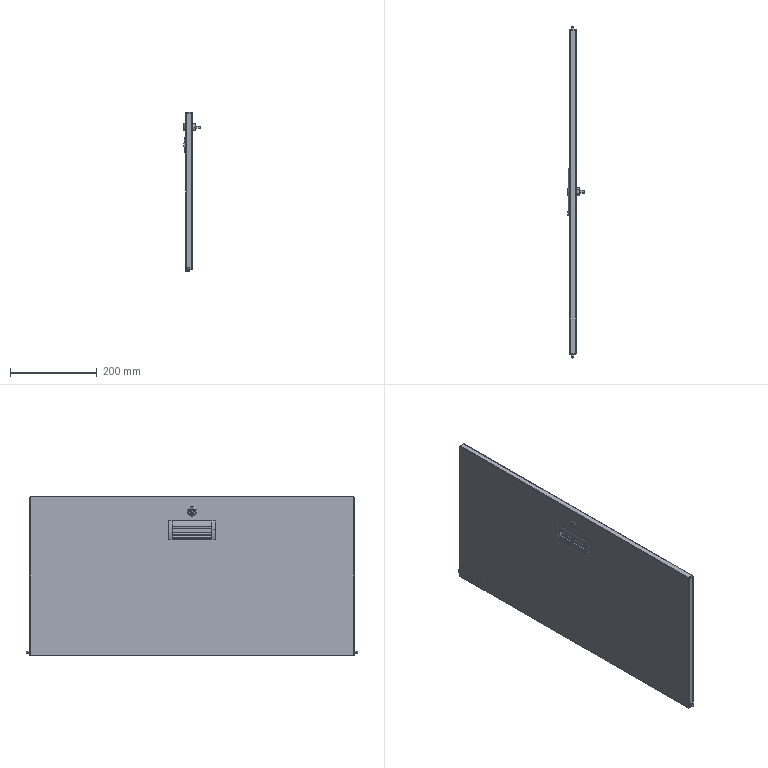Part | SolidWorks | 9 solids | 275 faces | box 37.5 x 764 x 367.5 mm | volume 509414 mm3 | plane 151 | cylinder 106 | spline 8 | cone 6 | torus 4 | commonest cylinder face diameters 1 x18 7 x10 5.5 x8 6 x8 0.6 x7 3.6 x7